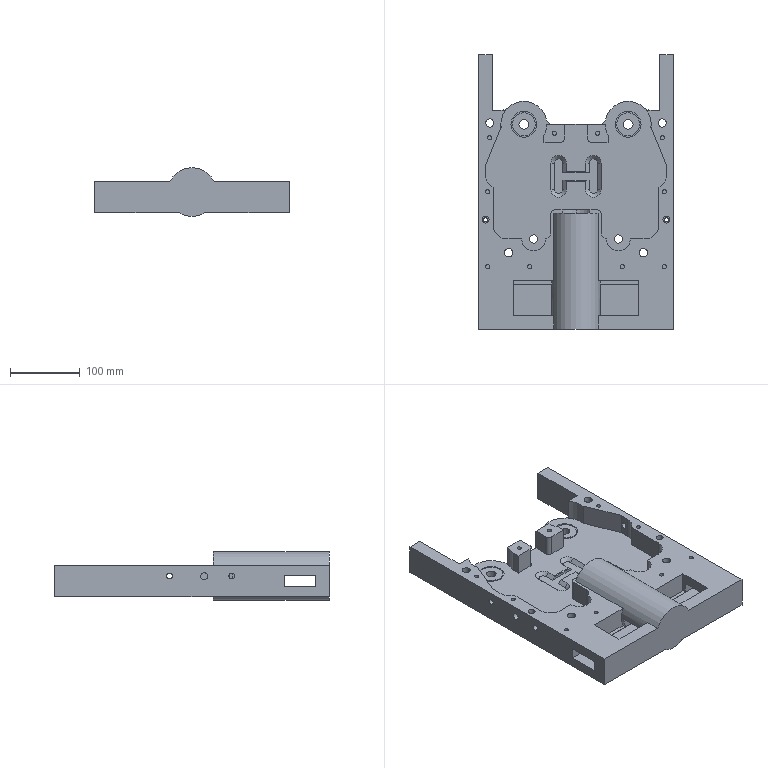Part | SolidWorks | features Attribute 187, ICE 26, Cut 11, Chamfer 4, Fillet 3, Extrusion 1, MirrorPattern 1 | 1 solid | 199 faces | box 280 x 394.673 x 70 mm | volume 2510782 mm3 | cylinder 104 | plane 91 | cone 4 | commonest cylinder face diameters 6 x24 12 x14 4 x10 10 x10 8.5 x8 66 x7